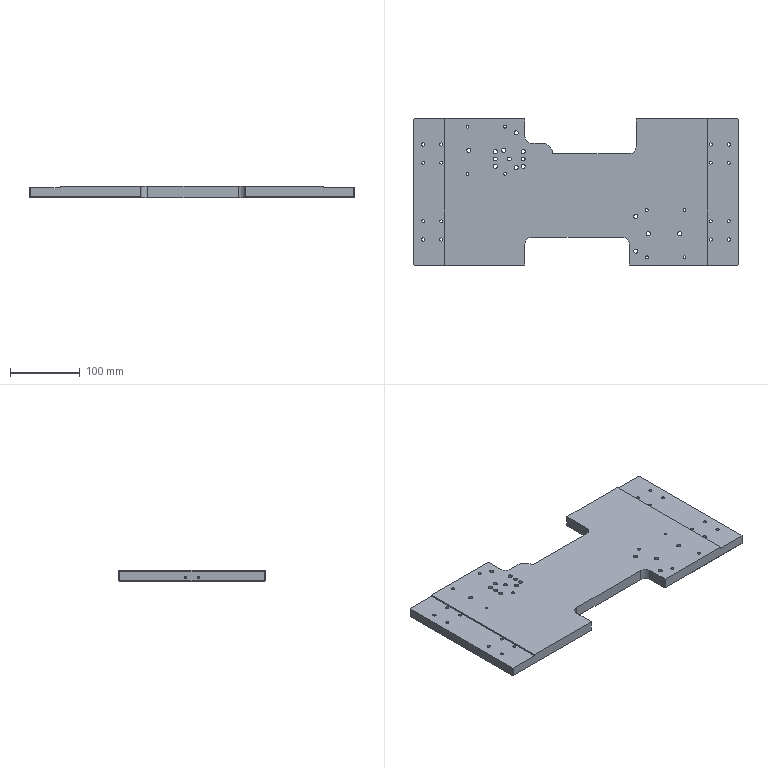NC program | NX | posted with a generic post | part box 467 x 210 x 16 mm
Whole program:
N10 G17 G21 G94 G90
(FLOOR_WALL_COPY , TOOL : D63)
N12 T01 M6
N14 G54
N16 G17 G0 G90 X-268. Y104.997 S6500 M3
N18 G43 Z30. H1
N20 Z3.
N22 G94 G1 Z0. F1250.
N24 X-265.
N26 X265.
N28 Y74.198
N30 X-265.
N32 Y43.398
N34 X265.
N36 Y12.599
N38 X-265.
N40 Y-18.201
N42 X265.
N44 Y-49.
N46 X-265.
N48 Y-75.229
N50 Y-79.8
N52 X265.
N54 X268.
N56 Z3.
N58 G0 Z30.
N60 M5
(CUTTER_COMP_11_COPY , TOOL : D10)
N62 T10 M6
N64 G54
N66 G17 G0 G90 X-240. Y-4.33 S7000 M3
N68 G43 Z30. H10
N70 Z0.5
N72 G94 G1 Z-1. F2000.
N74 X-234. Y-0.866
N76 G3 X-233.5 Y0. R1.
N78 G1 Y104.
N80 X-232.5 Y105.
N82 X-195.1
N84 Y-105.
N86 X-232.5
N88 X-233.5 Y-104.
N90 Y0.
N92 X-226.5
N94 Y98.
N96 X-202.1
N98 Y-98.
N100 X-226.5
N102 Y0.
N104 X-219.5
N106 Y91.
N108 X-209.1
N110 Y-91.
N112 X-219.5
N114 Y0.
N116 X-215.
N118 Y86.5
N120 X-213.6
N122 Y-86.5
N124 X-215.
N126 Y0.
N128 G3 X-215.5 Y0.866 R1.
N130 G1 Z0.5
N132 G0 Z3.
N134 G1 X-196.6 Y-103.5 F6000.
N136 G0 Z0.5
N138 G1 Z-1. F2000.
N140 X-195.1 Y-105.866
N142 G3 X-194.6 Y-105. R1.
N144 G1 Y105.
N146 G3 X-195.1 Y105.866 R1.
N148 G1 X-196.6 Y103.5
N150 Z0.5
N152 G0 Z3.
N154 G1 X-240. Y-4.33 F6000.
N156 G0 Z-0.5
N158 G1 Z-2. F2000.
N160 X-234. Y-0.866
N162 G3 X-233.5 Y0. R1.
N164 G1 Y104.
N166 X-232.5 Y105.
N168 X-195.1
N170 Y-105.
N172 X-232.5
N174 X-233.5 Y-104.
N176 Y0.
N178 X-226.5
N180 Y98.
N182 X-202.1
N184 Y-98.
N186 X-226.5
N188 Y0.
N190 X-219.5
N192 Y91.
N194 X-209.1
N196 Y-91.
N198 X-219.5
N200 Y0.
N202 X-215.
N204 Y86.5
N206 X-213.6
N208 Y-86.5
N210 X-215.
N212 Y0.
N214 G3 X-215.5 Y0.866 R1.
N216 G1 Z-0.5
N218 G0 Z2.
N220 G1 X-196.6 Y-103.5 F6000.
N222 G0 Z-0.5
N224 G1 Z-2. F2000.
N226 X-195.1 Y-105.866
N228 G3 X-194.6 Y-105. R1.
N230 G1 Y105.
N232 G3 X-195.1 Y105.866 R1.
N234 G1 X-196.6 Y103.5
N236 Z-0.5
N238 G0 Z30.
N240 X240. Y4.33
N242 Z0.5
N244 G1 Z-1.
N246 X234. Y0.866
N248 G3 X233.5 Y0. R1.
N250 G1 Y-104.
N252 X232.5 Y-105.
N254 X195.1
N256 Y105.
N258 X232.5
N260 X233.5 Y104.
N262 Y0.
N264 X226.5
N266 Y-98.
N268 X202.1
N270 Y98.
N272 X226.5
N274 Y0.
N276 X219.5
N278 Y-91.
N280 X209.1
N282 Y91.
N284 X219.5
N286 Y0.
N288 X215.
N290 Y-86.5
N292 X213.6
N294 Y86.5
N296 X215.
N298 Y0.
N300 G3 X215.5 Y-0.866 R1.
N302 G1 Z0.5
N304 G0 Z3.
N306 G1 X196.6 Y103.5 F6000.
N308 G0 Z0.5
N310 G1 Z-1. F2000.
N312 X195.1 Y105.866
N314 G3 X194.6 Y105. R1.
N316 G1 Y-105.
N318 G3 X195.1 Y-105.866 R1.
N320 G1 X196.6 Y-103.5
N322 Z0.5
N324 G0 Z3.
N326 G1 X240. Y4.33 F6000.
N328 G0 Z-0.5
N330 G1 Z-2. F2000.
N332 X234. Y0.866
N334 G3 X233.5 Y0. R1.
N336 G1 Y-104.
N338 X232.5 Y-105.
N340 X195.1
N342 Y105.
N344 X232.5
N346 X233.5 Y104.
N348 Y0.
N350 X226.5
N352 Y-98.
N354 X202.1
N356 Y98.
N358 X226.5
N360 Y0.
N362 X219.5
N364 Y-91.
N366 X209.1
N368 Y91.
N370 X219.5
N372 Y0.
N374 X215.
N376 Y-86.5
N378 X213.6
N380 Y86.5
N382 X215.
N384 Y0.
N386 G3 X215.5 Y-0.866 R1.
N388 G1 Z-0.5
N390 G0 Z2.
N392 G1 X196.6 Y103.5 F6000.
N394 G0 Z-0.5
N396 G1 Z-2. F2000.
N398 X195.1 Y105.866
N400 G3 X194.6 Y105. R1.
N402 G1 Y-105.
N404 G3 X195.1 Y-105.866 R1.
N406 G1 X196.6 Y-103.5
N408 Z-0.5
N410 G0 Z30.
N412 M5
(FLOOR_WALL_1_COPY_1 , TOOL : D10JING)
N414 T11 M6
N416 G54
N418 G17 G0 G90 X-239.479 Y-107.214 S7000 M3
N420 G43 Z30. H11
N422 Z-0.5
N424 G94 G1 Z-2. F1000.
N426 X-239. Y-106.937
N428 G3 X-238.5 Y-106.071 R1.
N430 G1 Y106.071
N432 X-234.571 Y110.
N434 X-233.667
N436 Y-110.
N438 X-228.833
N440 Y110.
N442 X-224.
N444 Y-110.
N446 X-219.167
N448 Y110.
N450 X-214.333
N452 Y-110.
N454 X-209.5
N456 Y110.
N458 X-204.667
N460 Y-110.
N462 X-199.833
N464 Y110.
N466 X-195.
N468 Y-110.
N470 G2 X-195.5 Y-110.866 R1.
N472 G1 X-196.598 Y-111.5
N474 Z-0.5
N476 G0 Z1.1
N478 G1 X-196.098 F6000.
N480 G0 Z-0.5
N482 G1 Z-2. F1000.
N484 X-195. Y-110.866
N486 G3 X-194.5 Y-110. R1.
N488 G1 Y110.
N490 G3 X-195. Y110.866 R1.
N492 G1 X-196.098 Y111.5
N494 Z-0.5
N496 G0 Z30.
N498 X239.479 Y107.214
N500 Z-0.5
N502 G1 Z-2.
N504 X239. Y106.937
N506 G3 X238.5 Y106.071 R1.
N508 G1 Y-106.071
N510 X234.571 Y-110.
N512 X233.667
N514 Y110.
N516 X228.833
N518 Y-110.
N520 X224.
N522 Y110.
N524 X219.167
N526 Y-110.
N528 X214.333
N530 Y110.
N532 X209.5
N534 Y-110.
N536 X204.667
N538 Y110.
N540 X199.833
N542 Y-110.
N544 X195.
N546 Y110.
N548 G2 X195.5 Y110.866 R1.
N550 G1 X196.598 Y111.5
N552 Z-0.5
N554 G0 Z1.1
N556 G1 X196.098 F6000.
N558 G0 Z-0.5
N560 G1 Z-2. F1000.
N562 X195. Y110.866
N564 G3 X194.5 Y110. R1.
N566 G1 Y-110.
N568 G3 X195. Y-110.866 R1.
N570 G1 X196.098 Y-111.5
N572 Z-0.5
N574 G0 Z30.
N576 M5
(ZLEVEL_PROFILE_COPY_1_COPY_COPY_COPY_COPY_2_COPY_1 , TOOL : D6A45)
N578 T07 M6
N580 G54
N582 G17 G0 G90 X-115.759 Y58.806 S7000 M3
N584 G43 Z30. H7
N586 Z-1.
N588 G94 G1 X-115.48 Y59.741 F1000.
N590 G3 X-116. Y60.041 R0.6
N592 G1 X-116.004
N594 G3 X-118.041 Y57.996 R2.041
N596 X-116. Y60.041 R-2.041
N598 X-116.52 Y59.741 R0.6
N600 G1 X-116.241 Y58.806
N602 G0 Z30.
N604 X-75.805 Y48.058
N606 Z-1.
N608 G1 X-75.48 Y48.991
N610 G3 X-76. Y49.291 R0.6
N612 G1 X-76.007
N614 G3 X-77.791 Y47.493 R1.791
N616 X-76. Y49.291 R-1.791
N618 X-76.52 Y48.991 R0.6
N620 G1 X-76.195 Y48.058
N622 G0 Z30.
N624 X-95.805
N626 Z-1.
N628 G1 X-95.48 Y48.991
N630 G3 X-96. Y49.291 R0.6
N632 G1 X-96.006
N634 G3 X-97.791 Y47.494 R1.791
N636 X-96. Y49.291 R-1.791
N638 X-96.52 Y48.991 R0.6
N640 G1 X-96.195 Y48.058
N642 G0 Z30.
N644 X-115.805
N646 Z-1.
N648 G1 X-115.48 Y48.991
N650 G3 X-116. Y49.291 R0.6
N652 G1 X-116.004
N654 G3 X-117.791 Y47.496 R1.791
N656 X-116. Y49.291 R-1.791
N658 X-116.52 Y48.991 R0.6
N660 G1 X-116.195 Y48.058
N662 G0 Z30.
N664 X-75.759 Y37.806
N666 Z-1.
N668 G1 X-75.48 Y38.741
N670 G3 X-76. Y39.041 R0.6
N672 G1 X-76.007
N674 G3 X-78.041 Y36.993 R2.041
N676 X-76. Y39.041 R-2.041
N678 X-76.52 Y38.741 R0.6
N680 G1 X-76.241 Y37.806
N682 G0 Z30.
N684 X-85.759 Y85.806
N686 Z-1.
N688 G1 X-85.48 Y86.741
N690 G3 X-86. Y87.041 R0.6
N692 X-88.041 Y85. R2.041
N694 X-86. Y87.041 R-2.041
N696 X-86.52 Y86.741 R0.6
N698 G1 X-86.241 Y85.806
N700 G0 Z30.
N702 X-115.759 Y37.806
N704 Z-1.
N706 G1 X-115.48 Y38.741
N708 G3 X-116. Y39.041 R0.6
N710 G1 X-116.004
N712 G3 X-118.041 Y36.996 R2.041
N714 X-116. Y39.041 R-2.041
N716 X-116.52 Y38.741 R0.6
N718 G1 X-116.241 Y37.806
N720 G0 Z30.
N722 X-85.759 Y35.806
N724 Z-1.
N726 G1 X-85.48 Y36.741
N728 G3 X-86. Y37.041 R0.6
N730 X-88.041 Y35. R2.041
N732 X-86. Y37.041 R-2.041
N734 X-86.52 Y36.741 R0.6
N736 G1 X-86.241 Y35.806
N738 G0 Z30.
N740 X-102. Y27.141
N742 Z0.
N744 G1 Z-1.
N746 X-102.003
N748 G3 X-103.141 Y25.997 R1.141
N750 X-102. Y27.141 R-1.141
N752 X-102.52 Y26.841 R0.6
N754 G0 Z30.
N756 X-157.141 Y26.
N758 Z0.
N760 G1 Z-1.
N762 G3 X-156. Y24.859 R1.141
N764 X-157.141 Y26. R-1.141
N766 X-156.841 Y25.48 R0.6
N768 G0 Z30.
N770 X157.141 Y-26.
N772 Z0.
N774 G1 Z-1.
N776 G3 X156. Y-24.859 R1.141
N778 X157.141 Y-26. R-1.141
N780 X156.841 Y-25.48 R0.6
N782 G0 Z30.
N784 X102. Y-27.141
N786 Z0.
N788 G1 Z-1.
N790 X102.003
N792 G3 X103.141 Y-25.997 R1.141
N794 X102. Y-27.141 R-1.141
N796 X102.52 Y-26.841 R0.6
N798 G0 Z30.
N800 X-156. Y95.141
N802 Z0.
N804 G1 Z-1.
N806 G3 X-157.141 Y94. R1.141
N808 X-156. Y95.141 R-1.141
N810 X-156.52 Y94.841 R0.6
N812 G0 Z30.
N814 X85.759 Y-35.806
N816 Z-1.
N818 G1 X85.48 Y-36.741
N820 G3 X86. Y-37.041 R0.6
N822 X88.041 Y-35. R2.041
N824 X86. Y-37.041 R-2.041
N826 X86.52 Y-36.741 R0.6
N828 G1 X86.241 Y-35.806
N830 G0 Z30.
N832 X-102. Y95.141
N834 Z0.
N836 G1 Z-1.
N838 X-102.003
N840 G3 X-103.141 Y93.997 R1.141
N842 X-102. Y95.141 R-1.141
N844 X-102.52 Y94.841 R0.6
N846 G0 Z30.
N848 X-103.759 Y60.806
N850 Z-1.
N852 G1 X-103.48 Y61.741
N854 G3 X-104. Y62.041 R0.6
N856 X-106.041 Y60. R2.041
N858 X-104. Y62.041 R-2.041
N860 X-104.52 Y61.741 R0.6
N862 G1 X-104.241 Y60.806
N864 G0 Z30.
N866 X148.759 Y-60.806
N868 Z-1.
N870 G1 X148.48 Y-61.741
N872 G3 X149. Y-62.041 R0.6
N874 X151.041 Y-60. R2.041
N876 X149. Y-62.041 R-2.041
N878 X149.52 Y-61.741 R0.6
N880 G1 X149.241 Y-60.806
N882 G0 Z30.
N884 X103.759
N886 Z-1.
N888 G1 X103.48 Y-61.741
N890 G3 X104. Y-62.041 R0.6
N892 X106.041 Y-60. R2.041
N894 X104. Y-62.041 R-2.041
N896 X104.52 Y-61.741 R0.6
N898 G1 X104.241 Y-60.806
N900 G0 Z30.
N902 X-153.759 Y60.806
N904 Z-1.
N906 G1 X-153.48 Y61.741
N908 G3 X-154. Y62.041 R0.6
N910 X-156.041 Y60. R2.041
N912 X-154. Y62.041 R-2.041
N914 X-154.52 Y61.741 R0.6
N916 G1 X-154.241 Y60.806
N918 G0 Z30.
N920 X85.759 Y-85.806
N922 Z-1.
N924 G1 X85.48 Y-86.741
N926 G3 X86. Y-87.041 R0.6
N928 X88.041 Y-85. R2.041
N930 X86. Y-87.041 R-2.041
N932 X86.52 Y-86.741 R0.6
N934 G1 X86.241 Y-85.806
N936 G0 Z30.
N938 X156. Y-95.141
N940 Z0.
N942 G1 Z-1.
N944 G3 X157.141 Y-94. R1.141
N946 X156. Y-95.141 R-1.141
N948 X156.52 Y-94.841 R0.6
N950 G0 Z30.
N952 X102. Y-95.141
N954 Z0.
N956 G1 Z-1.
N958 X102.003
N960 G3 X103.141 Y-93.997 R1.141
N962 X102. Y-95.141 R-1.141
N964 X102.52 Y-94.841 R0.6
N966 G0 Z30.
N968 X-75.759 Y58.806
N970 Z-1.
N972 G1 X-75.48 Y59.741
N974 G3 X-76. Y60.041 R0.6
N976 G1 X-76.007
N978 G3 X-78.041 Y57.993 R2.041
N980 X-76. Y60.041 R-2.041
N982 X-76.52 Y59.741 R0.6
N984 G1 X-76.241 Y58.806
N986 G0 Z30.
N988 X-191.453 Y-105.921
N990 Z-1.
N992 G1 X-190.759 Y-105.52
N994 G3 X-190.459 Y-105.001 R0.6
N996 G1 Y105.001
N998 G2 X-189.501 Y105.959 R0.958
N1000 G1 X-73.499
N1002 G2 X-72.541 Y105.001 R0.958
N1004 G1 Y80.
N1006 G3 X-63.5 Y70.959 R9.041
N1008 G1 X-43.499
N1010 G2 X-42.823 Y70.678 R0.957
N1012 G1 X-32.822 Y60.677
N1014 G2 X-32.541 Y60.002 R0.956
N1016 G1 Y55.959
N1018 X76.5
N1020 G3 X85.541 Y65. R9.041
N1022 G1 Y105.001
N1024 G2 X86.499 Y105.959 R0.958
N1026 G1 X189.501
N1028 G2 X190.459 Y105.001 R0.958
N1030 G1 Y-105.001
N1032 G2 X189.501 Y-105.959 R0.958
N1034 G1 X76.499
N1036 G2 X75.541 Y-105.001 R0.966
N1038 G1 Y-75.
N1040 G3 X66.5 Y-65.959 R9.041
N1042 G1 X-63.5
N1044 G3 X-72.541 Y-75. R9.041
N1046 G1 Y-105.001
N1048 G2 X-73.499 Y-105.959 R0.958
N1050 G1 X-189.501
N1052 G2 X-190.459 Y-105.001 R0.958
N1054 G3 X-190.759 Y-104.481 R0.6
N1056 G1 X-191.659 Y-103.962
N1058 G0 Z30.
(ZLEVEL_PROFILE_COPY_1_COPY_COPY_COPY_COPY_2_COPY_1_COPY , TOOL : D6A45)
N1060 X219.581 Y-42.342
N1062 Z-3.
N1064 G1 X220.491 Y-42.82
N1066 G3 X220.791 Y-42.3 R0.6
N1068 X219.5 Y-41.009 R1.291
N1070 X220.791 Y-42.3 R-1.291
N1072 X220.491 Y-41.78 R0.6
N1074 G1 X219.581 Y-42.258
N1076 G0 Z30.
N1078 X192.801 Y-43.386
N1080 Z-2.
N1082 G1 Z-3.
N1084 G3 X192.801 Y-41.214 R-1.291
N1086 X192.663 Y-41.481 R0.3
N1088 G0 Z30.
N1090 X-192.801 Y-41.214
N1092 Z-2.
N1094 G1 Z-3.
N1096 G3 X-192.801 Y-43.386 R-1.291
N1098 X-192.663 Y-43.119 R0.3
N1100 G0 Z30.
N1102 X-219.581 Y-42.258
N1104 Z-3.
N1106 G1 X-220.491 Y-41.78
N1108 G3 X-220.791 Y-42.3 R0.6
N1110 X-219.5 Y-43.591 R1.291
N1112 X-220.791 Y-42.3 R-1.291
N1114 X-220.491 Y-42.82 R0.6
N1116 G1 X-219.581 Y-42.342
N1118 G0 Z30.
N1120 X219.581 Y68.258
N1122 Z-3.
N1124 G1 X220.491 Y67.78
N1126 G3 X220.791 Y68.3 R0.6
N1128 X219.5 Y69.591 R1.291
N1130 X220.791 Y68.3 R-1.291
N1132 X220.491 Y68.82 R0.6
N1134 G1 X219.581 Y68.342
N1136 G0 Z30.
N1138 X192.801 Y67.214
N1140 Z-2.
N1142 G1 Z-3.
N1144 G3 X192.801 Y69.386 R-1.291
N1146 X192.663 Y69.119 R0.3
N1148 G0 Z30.
N1150 X219.581 Y42.258
N1152 Z-3.
N1154 G1 X220.491 Y41.78
N1156 G3 X220.791 Y42.3 R0.6
N1158 X219.5 Y43.591 R1.291
N1160 X220.791 Y42.3 R-1.291
N1162 X220.491 Y42.82 R0.6
N1164 G1 X219.581 Y42.342
N1166 G0 Z30.
N1168 Y-68.342
N1170 Z-3.
N1172 G1 X220.491 Y-68.82
N1174 G3 X220.791 Y-68.3 R0.6
N1176 X219.5 Y-67.009 R1.291
N1178 X220.791 Y-68.3 R-1.291
N1180 X220.491 Y-67.78 R0.6
N1182 G1 X219.581 Y-68.258
N1184 G0 Z30.
N1186 X192.801 Y-69.386
N1188 Z-2.
N1190 G1 Z-3.
N1192 G3 X192.801 Y-67.214 R-1.291
N1194 X192.664 Y-67.481 R0.3
N1196 G0 Z30.
N1198 X-192.801 Y-67.214
N1200 Z-2.
N1202 G1 Z-3.
N1204 G3 X-192.801 Y-69.386 R-1.291
N1206 X-192.663 Y-69.119 R0.3
N1208 G0 Z30.
N1210 X-219.581 Y-68.258
N1212 Z-3.
N1214 G1 X-220.491 Y-67.78
N1216 G3 X-220.791 Y-68.3 R0.6
N1218 X-219.5 Y-69.591 R1.291
N1220 X-220.791 Y-68.3 R-1.291
N1222 X-220.491 Y-68.82 R0.6
N1224 G1 X-219.581 Y-68.342
N1226 G0 Z30.
N1228 X-192.801 Y69.386
N1230 Z-2.
N1232 G1 Z-3.
N1234 G3 X-192.801 Y67.214 R-1.291
N1236 X-192.664 Y67.481 R0.3
N1238 G0 Z30.
N1240 X192.801 Y41.214
N1242 Z-2.
N1244 G1 Z-3.
N1246 G3 X192.801 Y43.386 R-1.291
N1248 X192.663 Y43.119 R0.3
N1250 G0 Z30.
N1252 X-192.801 Y43.386
N1254 Z-2.
N1256 G1 Z-3.
N1258 G3 X-192.801 Y41.214 R-1.291
N1260 X-192.663 Y41.481 R0.3
N1262 G0 Z30.
N1264 X-219.581 Y42.342
N1266 Z-3.
N1268 G1 X-220.491 Y42.82
N1270 G3 X-220.791 Y42.3 R0.6
N1272 X-219.5 Y41.009 R1.291
N1274 X-220.791 Y42.3 R-1.291
N1276 X-220.491 Y41.78 R0.6
N1278 G1 X-219.581 Y42.258
N1280 G0 Z30.
N1282 Y68.342
N1284 Z-3.
N1286 G1 X-220.491 Y68.82
N1288 G3 X-220.791 Y68.3 R0.6
N1290 X-219.5 Y67.009 R1.291
N1292 X-220.791 Y68.3 R-1.291
N1294 X-220.491 Y67.78 R0.6
N1296 G1 X-219.581 Y68.258
N1298 G0 Z30.
N1300 X193.021 Y107.159
N1302 Z-3.
N1304 G1 X192.408 Y106.109
N1306 G3 X192.667 Y105.959 R0.3
N1308 G1 X232.501
N1310 G2 X233.177 Y105.678 R0.956
N1312 G1 X234.178 Y104.677
N1314 G2 X234.459 Y104.001 R0.957
N1316 G1 Y-104.001
N1318 G2 X234.178 Y-104.677 R0.957
N1320 G1 X233.177 Y-105.678
N1322 G2 X232.501 Y-105.959 R0.956
N1324 G1 X192.667
N1326 G3 X192.408 Y-106.109 R0.3
N1328 G1 X193.02 Y-107.159
N1330 G0 Z30.
N1332 X-193.019
N1334 Z-3.
N1336 G1 X-192.408 Y-106.109
N1338 G3 X-192.667 Y-105.959 R0.3
N1340 G1 X-232.501
N1342 G2 X-233.177 Y-105.678 R0.956
N1344 G1 X-234.178 Y-104.677
N1346 G2 X-234.459 Y-104.001 R0.957
N1348 G1 Y104.001
N1350 G2 X-234.178 Y104.677 R0.957
N1352 G1 X-233.177 Y105.678
N1354 G2 X-232.501 Y105.959 R0.956
N1356 G1 X-192.667
N1358 G3 X-192.408 Y106.109 R0.3
N1360 G1 X-193.02 Y107.159
N1362 G0 Z30.
N1364 M5
N1366 M2